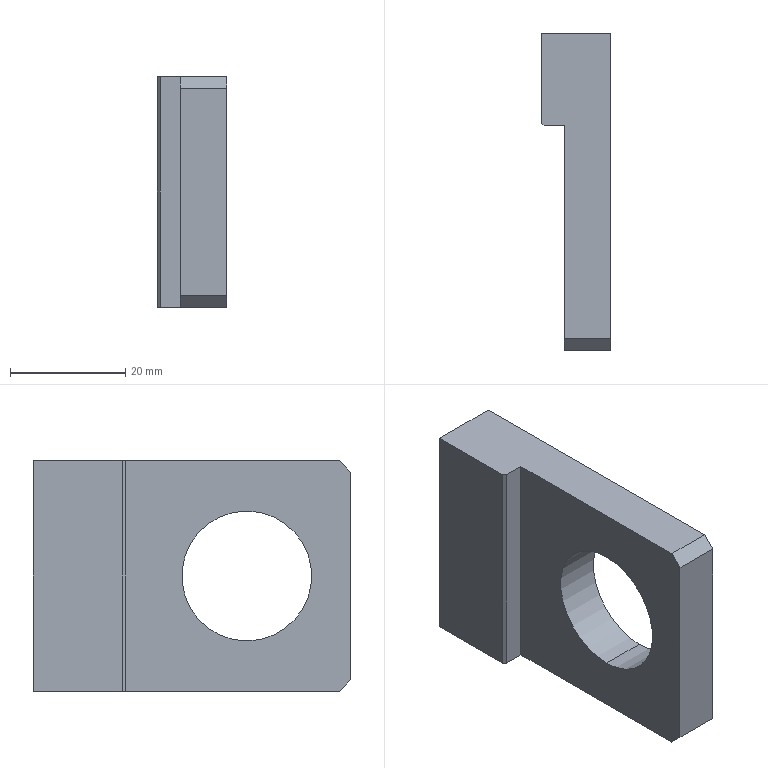Part | STEP file | PN_0027 | 1 solid | 21 faces | box 12 x 55 x 40 mm | volume 16587 mm3 | plane 11 | cylinder 6 | cone 4 | commonest cylinder face diameters 4.2 x4 22.5 x2
STEP:
#1=CARTESIAN_POINT('',(0.,0.,0.));
#2=DIRECTION('',(0.,0.,1.));
#3=DIRECTION('',(1.,0.,0.));
#4=AXIS2_PLACEMENT_3D('',#1,#2,#3);
#5=CARTESIAN_POINT('',(0.,-12.4,16.1));
#6=VERTEX_POINT('',#5);
#7=CARTESIAN_POINT('',(0.,0.,16.1));
#8=VERTEX_POINT('',#7);
#9=CARTESIAN_POINT('',(0.,0.,16.1));
#10=DIRECTION('',(0.,1.,0.));
#11=VECTOR('',#10,1.);
#12=LINE('',#9,#11);
#13=CARTESIAN_POINT('',(0.,0.,14.));
#14=DIRECTION('',(0.,1.,0.));
#15=DIRECTION('',(0.,0.,1.));
#16=AXIS2_PLACEMENT_3D('',#13,#14,#15);
#17=CYLINDRICAL_SURFACE('',#16,2.1);
#18=CARTESIAN_POINT('',(6.283,0.));
#19=DIRECTION('',(0.,1.));
#20=VECTOR('',#19,1.);
#21=LINE('',#18,#20);
#22=(GEOMETRIC_REPRESENTATION_CONTEXT(2)PARAMETRIC_REPRESENTATION_CONTEXT()REPRESENTATION_CONTEXT('',''));
#23=DEFINITIONAL_REPRESENTATION('',(#21),#22);
#24=PCURVE('',#17,#23);
#25=CARTESIAN_POINT('',(0.,0.,14.));
#26=DIRECTION('',(0.,1.,0.));
#27=DIRECTION('',(0.,0.,1.));
#28=AXIS2_PLACEMENT_3D('',#25,#26,#27);
#29=CYLINDRICAL_SURFACE('',#28,2.1);
#30=CARTESIAN_POINT('',(0.,0.));
#31=DIRECTION('',(0.,1.));
#32=VECTOR('',#31,1.);
#33=LINE('',#30,#32);
#34=(GEOMETRIC_REPRESENTATION_CONTEXT(2)PARAMETRIC_REPRESENTATION_CONTEXT()REPRESENTATION_CONTEXT('',''));
#35=DEFINITIONAL_REPRESENTATION('',(#33),#34);
#36=PCURVE('',#29,#35);
#37=SURFACE_CURVE('',#12,(#24,#36),.PCURVE_S1.);
#38=EDGE_CURVE('',#6,#8,#37,.T.);
#39=ORIENTED_EDGE('',*,*,#38,.T.);
#40=CARTESIAN_POINT('',(0.,0.,11.9));
#41=VERTEX_POINT('',#40);
#42=CARTESIAN_POINT('',(0.,0.,14.));
#43=DIRECTION('',(0.,1.,0.));
#44=DIRECTION('',(0.,0.,1.));
#45=AXIS2_PLACEMENT_3D('',#42,#43,#44);
#46=CIRCLE('',#45,2.1);
#47=CARTESIAN_POINT('',(0.,0.));
#48=DIRECTION('',(1.,0.));
#49=VECTOR('',#48,1.);
#50=LINE('',#47,#49);
#51=(GEOMETRIC_REPRESENTATION_CONTEXT(2)PARAMETRIC_REPRESENTATION_CONTEXT()REPRESENTATION_CONTEXT('',''));
#52=DEFINITIONAL_REPRESENTATION('',(#50),#51);
#53=PCURVE('',#17,#52);
#54=CARTESIAN_POINT('',(0.,0.,0.));
#55=DIRECTION('',(0.,1.,0.));
#56=DIRECTION('',(0.,0.,1.));
#57=AXIS2_PLACEMENT_3D('',#54,#55,#56);
#58=PLANE('',#57);
#59=CARTESIAN_POINT('',(14.,0.));
#60=DIRECTION('',(1.,0.));
#61=AXIS2_PLACEMENT_2D('',#59,#60);
#62=CIRCLE('',#61,2.1);
#63=(GEOMETRIC_REPRESENTATION_CONTEXT(2)PARAMETRIC_REPRESENTATION_CONTEXT()REPRESENTATION_CONTEXT('',''));
#64=DEFINITIONAL_REPRESENTATION('',(#62),#63);
#65=PCURVE('',#58,#64);
#66=SURFACE_CURVE('',#46,(#53,#65),.PCURVE_S1.);
#67=EDGE_CURVE('',#41,#8,#66,.T.);
#68=ORIENTED_EDGE('',*,*,#67,.F.);
#69=CARTESIAN_POINT('',(0.,-12.4,11.9));
#70=VERTEX_POINT('',#69);
#71=CARTESIAN_POINT('',(0.,0.,11.9));
#72=DIRECTION('',(0.,1.,0.));
#73=VECTOR('',#72,1.);
#74=LINE('',#71,#73);
#75=CARTESIAN_POINT('',(3.142,0.));
#76=DIRECTION('',(0.,1.));
#77=VECTOR('',#76,1.);
#78=LINE('',#75,#77);
#79=(GEOMETRIC_REPRESENTATION_CONTEXT(2)PARAMETRIC_REPRESENTATION_CONTEXT()REPRESENTATION_CONTEXT('',''));
#80=DEFINITIONAL_REPRESENTATION('',(#78),#79);
#81=PCURVE('',#17,#80);
#82=CARTESIAN_POINT('',(3.142,0.));
#83=DIRECTION('',(0.,1.));
#84=VECTOR('',#83,1.);
#85=LINE('',#82,#84);
#86=(GEOMETRIC_REPRESENTATION_CONTEXT(2)PARAMETRIC_REPRESENTATION_CONTEXT()REPRESENTATION_CONTEXT('',''));
#87=DEFINITIONAL_REPRESENTATION('',(#85),#86);
#88=PCURVE('',#29,#87);
#89=SURFACE_CURVE('',#74,(#81,#88),.PCURVE_S1.);
#90=EDGE_CURVE('',#70,#41,#89,.T.);
#91=ORIENTED_EDGE('',*,*,#90,.F.);
#92=CARTESIAN_POINT('',(0.,-12.4,14.));
#93=DIRECTION('',(0.,1.,0.));
#94=DIRECTION('',(0.,0.,1.));
#95=AXIS2_PLACEMENT_3D('',#92,#93,#94);
#96=CIRCLE('',#95,2.1);
#97=CARTESIAN_POINT('',(0.,-12.4));
#98=DIRECTION('',(1.,0.));
#99=VECTOR('',#98,1.);
#100=LINE('',#97,#99);
#101=(GEOMETRIC_REPRESENTATION_CONTEXT(2)PARAMETRIC_REPRESENTATION_CONTEXT()REPRESENTATION_CONTEXT('',''));
#102=DEFINITIONAL_REPRESENTATION('',(#100),#101);
#103=PCURVE('',#17,#102);
#104=CARTESIAN_POINT('',(0.,-12.4,14.));
#105=DIRECTION('',(0.,1.,0.));
#106=DIRECTION('',(0.,0.,1.));
#107=AXIS2_PLACEMENT_3D('',#104,#105,#106);
#108=CONICAL_SURFACE('',#107,2.1,1.03);
#109=CARTESIAN_POINT('',(0.,0.));
#110=DIRECTION('',(1.,0.));
#111=VECTOR('',#110,1.);
#112=LINE('',#109,#111);
#113=(GEOMETRIC_REPRESENTATION_CONTEXT(2)PARAMETRIC_REPRESENTATION_CONTEXT()REPRESENTATION_CONTEXT('',''));
#114=DEFINITIONAL_REPRESENTATION('',(#112),#113);
#115=PCURVE('',#108,#114);
#116=SURFACE_CURVE('',#96,(#103,#115),.PCURVE_S1.);
#117=EDGE_CURVE('',#70,#6,#116,.T.);
#118=ORIENTED_EDGE('',*,*,#117,.T.);
#119=EDGE_LOOP('',(#39,#68,#91,#118));
#120=FACE_BOUND('',#119,.F.);
#121=ADVANCED_FACE('',(#120),#17,.F.);
#122=ORIENTED_EDGE('',*,*,#117,.F.);
#123=CARTESIAN_POINT('',(0.,-13.662,14.));
#124=VERTEX_POINT('',#123);
#125=CARTESIAN_POINT('',(0.,-12.4,11.9));
#126=DIRECTION('',(0.,0.515,-0.8572));
#127=VECTOR('',#126,1.);
#128=LINE('',#125,#127);
#129=CARTESIAN_POINT('',(3.142,0.));
#130=DIRECTION('',(0.,1.));
#131=VECTOR('',#130,1.);
#132=LINE('',#129,#131);
#133=(GEOMETRIC_REPRESENTATION_CONTEXT(2)PARAMETRIC_REPRESENTATION_CONTEXT()REPRESENTATION_CONTEXT('',''));
#134=DEFINITIONAL_REPRESENTATION('',(#132),#133);
#135=PCURVE('',#108,#134);
#136=CARTESIAN_POINT('',(0.,-12.4,14.));
#137=DIRECTION('',(0.,1.,0.));
#138=DIRECTION('',(0.,0.,1.));
#139=AXIS2_PLACEMENT_3D('',#136,#137,#138);
#140=CONICAL_SURFACE('',#139,2.1,1.03);
#141=CARTESIAN_POINT('',(3.142,0.));
#142=DIRECTION('',(0.,1.));
#143=VECTOR('',#142,1.);
#144=LINE('',#141,#143);
#145=(GEOMETRIC_REPRESENTATION_CONTEXT(2)PARAMETRIC_REPRESENTATION_CONTEXT()REPRESENTATION_CONTEXT('',''));
#146=DEFINITIONAL_REPRESENTATION('',(#144),#145);
#147=PCURVE('',#140,#146);
#148=SURFACE_CURVE('',#128,(#135,#147),.PCURVE_S1.);
#149=EDGE_CURVE('',#124,#70,#148,.T.);
#150=ORIENTED_EDGE('',*,*,#149,.F.);
#151=CARTESIAN_POINT('',(0.,-12.4,16.1));
#152=DIRECTION('',(0.,0.515,0.8572));
#153=VECTOR('',#152,1.);
#154=LINE('',#151,#153);
#155=CARTESIAN_POINT('',(6.283,0.));
#156=DIRECTION('',(0.,1.));
#157=VECTOR('',#156,1.);
#158=LINE('',#155,#157);
#159=(GEOMETRIC_REPRESENTATION_CONTEXT(2)PARAMETRIC_REPRESENTATION_CONTEXT()REPRESENTATION_CONTEXT('',''));
#160=DEFINITIONAL_REPRESENTATION('',(#158),#159);
#161=PCURVE('',#108,#160);
#162=CARTESIAN_POINT('',(0.,0.));
#163=DIRECTION('',(0.,1.));
#164=VECTOR('',#163,1.);
#165=LINE('',#162,#164);
#166=(GEOMETRIC_REPRESENTATION_CONTEXT(2)PARAMETRIC_REPRESENTATION_CONTEXT()REPRESENTATION_CONTEXT('',''));
#167=DEFINITIONAL_REPRESENTATION('',(#165),#166);
#168=PCURVE('',#140,#167);
#169=SURFACE_CURVE('',#154,(#161,#168),.PCURVE_S1.);
#170=EDGE_CURVE('',#124,#6,#169,.T.);
#171=ORIENTED_EDGE('',*,*,#170,.T.);
#172=EDGE_LOOP('',(#122,#150,#171));
#173=FACE_BOUND('',#172,.F.);
#174=ADVANCED_FACE('',(#173),#108,.F.);
#175=CARTESIAN_POINT('',(0.,-12.4,-11.9));
#176=VERTEX_POINT('',#175);
#177=CARTESIAN_POINT('',(0.,0.,-11.9));
#178=VERTEX_POINT('',#177);
#179=CARTESIAN_POINT('',(0.,0.,-11.9));
#180=DIRECTION('',(0.,1.,0.));
#181=VECTOR('',#180,1.);
#182=LINE('',#179,#181);
#183=CARTESIAN_POINT('',(0.,0.,-14.));
#184=DIRECTION('',(0.,1.,0.));
#185=DIRECTION('',(0.,0.,1.));
#186=AXIS2_PLACEMENT_3D('',#183,#184,#185);
#187=CYLINDRICAL_SURFACE('',#186,2.1);
#188=CARTESIAN_POINT('',(6.283,0.));
#189=DIRECTION('',(0.,1.));
#190=VECTOR('',#189,1.);
#191=LINE('',#188,#190);
#192=(GEOMETRIC_REPRESENTATION_CONTEXT(2)PARAMETRIC_REPRESENTATION_CONTEXT()REPRESENTATION_CONTEXT('',''));
#193=DEFINITIONAL_REPRESENTATION('',(#191),#192);
#194=PCURVE('',#187,#193);
#195=CARTESIAN_POINT('',(0.,0.,-14.));
#196=DIRECTION('',(0.,1.,0.));
#197=DIRECTION('',(0.,0.,1.));
#198=AXIS2_PLACEMENT_3D('',#195,#196,#197);
#199=CYLINDRICAL_SURFACE('',#198,2.1);
#200=CARTESIAN_POINT('',(0.,0.));
#201=DIRECTION('',(0.,1.));
#202=VECTOR('',#201,1.);
#203=LINE('',#200,#202);
#204=(GEOMETRIC_REPRESENTATION_CONTEXT(2)PARAMETRIC_REPRESENTATION_CONTEXT()REPRESENTATION_CONTEXT('',''));
#205=DEFINITIONAL_REPRESENTATION('',(#203),#204);
#206=PCURVE('',#199,#205);
#207=SURFACE_CURVE('',#182,(#194,#206),.PCURVE_S1.);
#208=EDGE_CURVE('',#176,#178,#207,.T.);
#209=ORIENTED_EDGE('',*,*,#208,.T.);
#210=CARTESIAN_POINT('',(0.,0.,-16.1));
#211=VERTEX_POINT('',#210);
#212=CARTESIAN_POINT('',(0.,0.,-14.));
#213=DIRECTION('',(0.,1.,0.));
#214=DIRECTION('',(0.,0.,1.));
#215=AXIS2_PLACEMENT_3D('',#212,#213,#214);
#216=CIRCLE('',#215,2.1);
#217=CARTESIAN_POINT('',(0.,0.));
#218=DIRECTION('',(1.,0.));
#219=VECTOR('',#218,1.);
#220=LINE('',#217,#219);
#221=(GEOMETRIC_REPRESENTATION_CONTEXT(2)PARAMETRIC_REPRESENTATION_CONTEXT()REPRESENTATION_CONTEXT('',''));
#222=DEFINITIONAL_REPRESENTATION('',(#220),#221);
#223=PCURVE('',#187,#222);
#224=CARTESIAN_POINT('',(-14.,0.));
#225=DIRECTION('',(1.,0.));
#226=AXIS2_PLACEMENT_2D('',#224,#225);
#227=CIRCLE('',#226,2.1);
#228=(GEOMETRIC_REPRESENTATION_CONTEXT(2)PARAMETRIC_REPRESENTATION_CONTEXT()REPRESENTATION_CONTEXT('',''));
#229=DEFINITIONAL_REPRESENTATION('',(#227),#228);
#230=PCURVE('',#58,#229);
#231=SURFACE_CURVE('',#216,(#223,#230),.PCURVE_S1.);
#232=EDGE_CURVE('',#211,#178,#231,.T.);
#233=ORIENTED_EDGE('',*,*,#232,.F.);
#234=CARTESIAN_POINT('',(0.,-12.4,-16.1));
#235=VERTEX_POINT('',#234);
#236=CARTESIAN_POINT('',(0.,0.,-16.1));
#237=DIRECTION('',(0.,1.,0.));
#238=VECTOR('',#237,1.);
#239=LINE('',#236,#238);
#240=CARTESIAN_POINT('',(3.142,0.));
#241=DIRECTION('',(0.,1.));
#242=VECTOR('',#241,1.);
#243=LINE('',#240,#242);
#244=(GEOMETRIC_REPRESENTATION_CONTEXT(2)PARAMETRIC_REPRESENTATION_CONTEXT()REPRESENTATION_CONTEXT('',''));
#245=DEFINITIONAL_REPRESENTATION('',(#243),#244);
#246=PCURVE('',#187,#245);
#247=CARTESIAN_POINT('',(3.142,0.));
#248=DIRECTION('',(0.,1.));
#249=VECTOR('',#248,1.);
#250=LINE('',#247,#249);
#251=(GEOMETRIC_REPRESENTATION_CONTEXT(2)PARAMETRIC_REPRESENTATION_CONTEXT()REPRESENTATION_CONTEXT('',''));
#252=DEFINITIONAL_REPRESENTATION('',(#250),#251);
#253=PCURVE('',#199,#252);
#254=SURFACE_CURVE('',#239,(#246,#253),.PCURVE_S1.);
#255=EDGE_CURVE('',#235,#211,#254,.T.);
#256=ORIENTED_EDGE('',*,*,#255,.F.);
#257=CARTESIAN_POINT('',(0.,-12.4,-14.));
#258=DIRECTION('',(0.,1.,0.));
#259=DIRECTION('',(0.,0.,1.));
#260=AXIS2_PLACEMENT_3D('',#257,#258,#259);
#261=CIRCLE('',#260,2.1);
#262=CARTESIAN_POINT('',(0.,-12.4));
#263=DIRECTION('',(1.,0.));
#264=VECTOR('',#263,1.);
#265=LINE('',#262,#264);
#266=(GEOMETRIC_REPRESENTATION_CONTEXT(2)PARAMETRIC_REPRESENTATION_CONTEXT()REPRESENTATION_CONTEXT('',''));
#267=DEFINITIONAL_REPRESENTATION('',(#265),#266);
#268=PCURVE('',#187,#267);
#269=CARTESIAN_POINT('',(0.,-12.4,-14.));
#270=DIRECTION('',(0.,1.,0.));
#271=DIRECTION('',(0.,0.,1.));
#272=AXIS2_PLACEMENT_3D('',#269,#270,#271);
#273=CONICAL_SURFACE('',#272,2.1,1.03);
#274=CARTESIAN_POINT('',(0.,0.));
#275=DIRECTION('',(1.,0.));
#276=VECTOR('',#275,1.);
#277=LINE('',#274,#276);
#278=(GEOMETRIC_REPRESENTATION_CONTEXT(2)PARAMETRIC_REPRESENTATION_CONTEXT()REPRESENTATION_CONTEXT('',''));
#279=DEFINITIONAL_REPRESENTATION('',(#277),#278);
#280=PCURVE('',#273,#279);
#281=SURFACE_CURVE('',#261,(#268,#280),.PCURVE_S1.);
#282=EDGE_CURVE('',#235,#176,#281,.T.);
#283=ORIENTED_EDGE('',*,*,#282,.T.);
#284=EDGE_LOOP('',(#209,#233,#256,#283));
#285=FACE_BOUND('',#284,.F.);
#286=ADVANCED_FACE('',(#285),#187,.F.);
#287=ORIENTED_EDGE('',*,*,#282,.F.);
#288=CARTESIAN_POINT('',(0.,-13.662,-14.));
#289=VERTEX_POINT('',#288);
#290=CARTESIAN_POINT('',(0.,-12.4,-16.1));
#291=DIRECTION('',(0.,0.515,-0.8572));
#292=VECTOR('',#291,1.);
#293=LINE('',#290,#292);
#294=CARTESIAN_POINT('',(3.142,0.));
#295=DIRECTION('',(0.,1.));
#296=VECTOR('',#295,1.);
#297=LINE('',#294,#296);
#298=(GEOMETRIC_REPRESENTATION_CONTEXT(2)PARAMETRIC_REPRESENTATION_CONTEXT()REPRESENTATION_CONTEXT('',''));
#299=DEFINITIONAL_REPRESENTATION('',(#297),#298);
#300=PCURVE('',#273,#299);
#301=CARTESIAN_POINT('',(0.,-12.4,-14.));
#302=DIRECTION('',(0.,1.,0.));
#303=DIRECTION('',(0.,0.,1.));
#304=AXIS2_PLACEMENT_3D('',#301,#302,#303);
#305=CONICAL_SURFACE('',#304,2.1,1.03);
#306=CARTESIAN_POINT('',(3.142,0.));
#307=DIRECTION('',(0.,1.));
#308=VECTOR('',#307,1.);
#309=LINE('',#306,#308);
#310=(GEOMETRIC_REPRESENTATION_CONTEXT(2)PARAMETRIC_REPRESENTATION_CONTEXT()REPRESENTATION_CONTEXT('',''));
#311=DEFINITIONAL_REPRESENTATION('',(#309),#310);
#312=PCURVE('',#305,#311);
#313=SURFACE_CURVE('',#293,(#300,#312),.PCURVE_S1.);
#314=EDGE_CURVE('',#289,#235,#313,.T.);
#315=ORIENTED_EDGE('',*,*,#314,.F.);
#316=CARTESIAN_POINT('',(0.,-12.4,-11.9));
#317=DIRECTION('',(0.,0.515,0.8572));
#318=VECTOR('',#317,1.);
#319=LINE('',#316,#318);
#320=CARTESIAN_POINT('',(6.283,0.));
#321=DIRECTION('',(0.,1.));
#322=VECTOR('',#321,1.);
#323=LINE('',#320,#322);
#324=(GEOMETRIC_REPRESENTATION_CONTEXT(2)PARAMETRIC_REPRESENTATION_CONTEXT()REPRESENTATION_CONTEXT('',''));
#325=DEFINITIONAL_REPRESENTATION('',(#323),#324);
#326=PCURVE('',#273,#325);
#327=CARTESIAN_POINT('',(0.,0.));
#328=DIRECTION('',(0.,1.));
#329=VECTOR('',#328,1.);
#330=LINE('',#327,#329);
#331=(GEOMETRIC_REPRESENTATION_CONTEXT(2)PARAMETRIC_REPRESENTATION_CONTEXT()REPRESENTATION_CONTEXT('',''));
#332=DEFINITIONAL_REPRESENTATION('',(#330),#331);
#333=PCURVE('',#305,#332);
#334=SURFACE_CURVE('',#319,(#326,#333),.PCURVE_S1.);
#335=EDGE_CURVE('',#289,#176,#334,.T.);
#336=ORIENTED_EDGE('',*,*,#335,.T.);
#337=EDGE_LOOP('',(#287,#315,#336));
#338=FACE_BOUND('',#337,.F.);
#339=ADVANCED_FACE('',(#338),#273,.F.);
#340=CARTESIAN_POINT('',(-2.,-37.,-11.25));
#341=VERTEX_POINT('',#340);
#342=CARTESIAN_POINT('',(6.,-37.,-11.25));
#343=VERTEX_POINT('',#342);
#344=CARTESIAN_POINT('',(-6.,-37.,-11.25));
#345=DIRECTION('',(1.,0.,0.));
#346=VECTOR('',#345,1.);
#347=LINE('',#344,#346);
#348=CARTESIAN_POINT('',(-6.,-37.,0.));
#349=DIRECTION('',(1.,0.,0.));
#350=DIRECTION('',(0.,0.,-1.));
#351=AXIS2_PLACEMENT_3D('',#348,#349,#350);
#352=CYLINDRICAL_SURFACE('',#351,11.25);
#353=CARTESIAN_POINT('',(6.283,0.));
#354=DIRECTION('',(0.,1.));
#355=VECTOR('',#354,1.);
#356=LINE('',#353,#355);
#357=(GEOMETRIC_REPRESENTATION_CONTEXT(2)PARAMETRIC_REPRESENTATION_CONTEXT()REPRESENTATION_CONTEXT('',''));
#358=DEFINITIONAL_REPRESENTATION('',(#356),#357);
#359=PCURVE('',#352,#358);
#360=CARTESIAN_POINT('',(-6.,-37.,0.));
#361=DIRECTION('',(1.,0.,0.));
#362=DIRECTION('',(0.,0.,-1.));
#363=AXIS2_PLACEMENT_3D('',#360,#361,#362);
#364=CYLINDRICAL_SURFACE('',#363,11.25);
#365=CARTESIAN_POINT('',(0.,0.));
#366=DIRECTION('',(0.,1.));
#367=VECTOR('',#366,1.);
#368=LINE('',#365,#367);
#369=(GEOMETRIC_REPRESENTATION_CONTEXT(2)PARAMETRIC_REPRESENTATION_CONTEXT()REPRESENTATION_CONTEXT('',''));
#370=DEFINITIONAL_REPRESENTATION('',(#368),#369);
#371=PCURVE('',#364,#370);
#372=SURFACE_CURVE('',#347,(#359,#371),.PCURVE_S1.);
#373=EDGE_CURVE('',#341,#343,#372,.T.);
#374=ORIENTED_EDGE('',*,*,#373,.T.);
#375=CARTESIAN_POINT('',(6.,-37.,11.25));
#376=VERTEX_POINT('',#375);
#377=CARTESIAN_POINT('',(6.,-37.,0.));
#378=DIRECTION('',(1.,0.,0.));
#379=DIRECTION('',(0.,0.,-1.));
#380=AXIS2_PLACEMENT_3D('',#377,#378,#379);
#381=CIRCLE('',#380,11.25);
#382=CARTESIAN_POINT('',(0.,12.));
#383=DIRECTION('',(1.,0.));
#384=VECTOR('',#383,1.);
#385=LINE('',#382,#384);
#386=(GEOMETRIC_REPRESENTATION_CONTEXT(2)PARAMETRIC_REPRESENTATION_CONTEXT()REPRESENTATION_CONTEXT('',''));
#387=DEFINITIONAL_REPRESENTATION('',(#385),#386);
#388=PCURVE('',#352,#387);
#389=CARTESIAN_POINT('',(6.,-55.,-20.));
#390=DIRECTION('',(1.,0.,0.));
#391=DIRECTION('',(0.,0.,-1.));
#392=AXIS2_PLACEMENT_3D('',#389,#390,#391);
#393=PLANE('',#392);
#394=CARTESIAN_POINT('',(-20.,18.));
#395=DIRECTION('',(1.,0.));
#396=AXIS2_PLACEMENT_2D('',#394,#395);
#397=CIRCLE('',#396,11.25);
#398=(GEOMETRIC_REPRESENTATION_CONTEXT(2)PARAMETRIC_REPRESENTATION_CONTEXT()REPRESENTATION_CONTEXT('',''));
#399=DEFINITIONAL_REPRESENTATION('',(#397),#398);
#400=PCURVE('',#393,#399);
#401=SURFACE_CURVE('',#381,(#388,#400),.PCURVE_S1.);
#402=EDGE_CURVE('',#376,#343,#401,.T.);
#403=ORIENTED_EDGE('',*,*,#402,.F.);
#404=CARTESIAN_POINT('',(-2.,-37.,11.25));
#405=VERTEX_POINT('',#404);
#406=CARTESIAN_POINT('',(-6.,-37.,11.25));
#407=DIRECTION('',(1.,0.,0.));
#408=VECTOR('',#407,1.);
#409=LINE('',#406,#408);
#410=CARTESIAN_POINT('',(3.142,0.));
#411=DIRECTION('',(0.,1.));
#412=VECTOR('',#411,1.);
#413=LINE('',#410,#412);
#414=(GEOMETRIC_REPRESENTATION_CONTEXT(2)PARAMETRIC_REPRESENTATION_CONTEXT()REPRESENTATION_CONTEXT('',''));
#415=DEFINITIONAL_REPRESENTATION('',(#413),#414);
#416=PCURVE('',#352,#415);
#417=CARTESIAN_POINT('',(3.142,0.));
#418=DIRECTION('',(0.,1.));
#419=VECTOR('',#418,1.);
#420=LINE('',#417,#419);
#421=(GEOMETRIC_REPRESENTATION_CONTEXT(2)PARAMETRIC_REPRESENTATION_CONTEXT()REPRESENTATION_CONTEXT('',''));
#422=DEFINITIONAL_REPRESENTATION('',(#420),#421);
#423=PCURVE('',#364,#422);
#424=SURFACE_CURVE('',#409,(#416,#423),.PCURVE_S1.);
#425=EDGE_CURVE('',#405,#376,#424,.T.);
#426=ORIENTED_EDGE('',*,*,#425,.F.);
#427=CARTESIAN_POINT('',(-2.,-37.,0.));
#428=DIRECTION('',(-1.,0.,0.));
#429=DIRECTION('',(0.,0.,-1.));
#430=AXIS2_PLACEMENT_3D('',#427,#428,#429);
#431=CIRCLE('',#430,11.25);
#432=CARTESIAN_POINT('',(6.283,4.));
#433=DIRECTION('',(-1.,0.));
#434=VECTOR('',#433,1.);
#435=LINE('',#432,#434);
#436=(GEOMETRIC_REPRESENTATION_CONTEXT(2)PARAMETRIC_REPRESENTATION_CONTEXT()REPRESENTATION_CONTEXT('',''));
#437=DEFINITIONAL_REPRESENTATION('',(#435),#436);
#438=PCURVE('',#352,#437);
#439=CARTESIAN_POINT('',(-2.,-55.,-20.));
#440=DIRECTION('',(1.,0.,0.));
#441=DIRECTION('',(0.,0.,-1.));
#442=AXIS2_PLACEMENT_3D('',#439,#440,#441);
#443=PLANE('',#442);
#444=CARTESIAN_POINT('',(-8.75,18.));
#445=CARTESIAN_POINT('',(-8.75,-1.486));
#446=CARTESIAN_POINT('',(-25.625,8.257));
#447=CARTESIAN_POINT('',(-42.5,18.));
#448=CARTESIAN_POINT('',(-25.625,27.743));
#449=CARTESIAN_POINT('',(-8.75,37.486));
#450=CARTESIAN_POINT('',(-8.75,18.));
#451=(BOUNDED_CURVE()B_SPLINE_CURVE(2,(#444,#445,#446,#447,#448,#449,#450),.UNSPECIFIED.,.T.,.F.)B_SPLINE_CURVE_WITH_KNOTS((1,2,2,2,2,1),(-2.094,0.,2.094,4.189,6.283,8.378),.UNSPECIFIED.)CURVE()GEOMETRIC_REPRESENTATION_ITEM()RATIONAL_B_SPLINE_CURVE((1.,0.5,1.,0.5,1.,0.5,1.))REPRESENTATION_ITEM(''));
#452=(GEOMETRIC_REPRESENTATION_CONTEXT(2)PARAMETRIC_REPRESENTATION_CONTEXT()REPRESENTATION_CONTEXT('',''));
#453=DEFINITIONAL_REPRESENTATION('',(#451),#452);
#454=PCURVE('',#443,#453);
#455=SURFACE_CURVE('',#431,(#438,#454),.PCURVE_S1.);
#456=EDGE_CURVE('',#341,#405,#455,.T.);
#457=ORIENTED_EDGE('',*,*,#456,.F.);
#458=EDGE_LOOP('',(#374,#403,#426,#457));
#459=FACE_BOUND('',#458,.F.);
#460=ADVANCED_FACE('',(#459),#352,.F.);
#461=CARTESIAN_POINT('',(6.,-37.,0.));
#462=DIRECTION('',(1.,0.,0.));
#463=DIRECTION('',(0.,0.,-1.));
#464=AXIS2_PLACEMENT_3D('',#461,#462,#463);
#465=CIRCLE('',#464,11.25);
#466=CARTESIAN_POINT('',(-20.,18.));
#467=DIRECTION('',(1.,0.));
#468=AXIS2_PLACEMENT_2D('',#466,#467);
#469=CIRCLE('',#468,11.25);
#470=(GEOMETRIC_REPRESENTATION_CONTEXT(2)PARAMETRIC_REPRESENTATION_CONTEXT()REPRESENTATION_CONTEXT('',''));
#471=DEFINITIONAL_REPRESENTATION('',(#469),#470);
#472=PCURVE('',#393,#471);
#473=CARTESIAN_POINT('',(0.,12.));
#474=DIRECTION('',(1.,0.));
#475=VECTOR('',#474,1.);
#476=LINE('',#473,#475);
#477=(GEOMETRIC_REPRESENTATION_CONTEXT(2)PARAMETRIC_REPRESENTATION_CONTEXT()REPRESENTATION_CONTEXT('',''));
#478=DEFINITIONAL_REPRESENTATION('',(#476),#477);
#479=PCURVE('',#364,#478);
#480=SURFACE_CURVE('',#465,(#472,#479),.PCURVE_S1.);
#481=EDGE_CURVE('',#343,#376,#480,.T.);
#482=ORIENTED_EDGE('',*,*,#481,.F.);
#483=ORIENTED_EDGE('',*,*,#402,.F.);
#484=EDGE_LOOP('',(#482,#483));
#485=FACE_BOUND('',#484,.T.);
#486=CARTESIAN_POINT('',(6.,-55.,18.));
#487=VERTEX_POINT('',#486);
#488=CARTESIAN_POINT('',(6.,-55.,-18.));
#489=VERTEX_POINT('',#488);
#490=CARTESIAN_POINT('',(6.,-55.,-20.));
#491=DIRECTION('',(0.,0.,-1.));
#492=VECTOR('',#491,1.);
#493=LINE('',#490,#492);
#494=CARTESIAN_POINT('',(0.,0.));
#495=DIRECTION('',(1.,0.));
#496=VECTOR('',#495,1.);
#497=LINE('',#494,#496);
#498=(GEOMETRIC_REPRESENTATION_CONTEXT(2)PARAMETRIC_REPRESENTATION_CONTEXT()REPRESENTATION_CONTEXT('',''));
#499=DEFINITIONAL_REPRESENTATION('',(#497),#498);
#500=PCURVE('',#393,#499);
#501=CARTESIAN_POINT('',(0.,-55.,0.));
#502=DIRECTION('',(0.,1.,0.));
#503=DIRECTION('',(0.,0.,1.));
#504=AXIS2_PLACEMENT_3D('',#501,#502,#503);
#505=PLANE('',#504);
#506=CARTESIAN_POINT('',(-20.,6.));
#507=DIRECTION('',(-1.,0.));
#508=VECTOR('',#507,1.);
#509=LINE('',#506,#508);
#510=(GEOMETRIC_REPRESENTATION_CONTEXT(2)PARAMETRIC_REPRESENTATION_CONTEXT()REPRESENTATION_CONTEXT('',''));
#511=DEFINITIONAL_REPRESENTATION('',(#509),#510);
#512=PCURVE('',#505,#511);
#513=SURFACE_CURVE('',#493,(#500,#512),.PCURVE_S1.);
#514=EDGE_CURVE('',#487,#489,#513,.T.);
#515=ORIENTED_EDGE('',*,*,#514,.T.);
#516=CARTESIAN_POINT('',(6.,-53.,-20.));
#517=VERTEX_POINT('',#516);
#518=CARTESIAN_POINT('',(6.,-54.,-19.));
#519=DIRECTION('',(0.,0.7071,-0.7071));
#520=VECTOR('',#519,1.);
#521=LINE('',#518,#520);
#522=CARTESIAN_POINT('',(-1.,1.));
#523=DIRECTION('',(0.7071,0.7071));
#524=VECTOR('',#523,1.);
#525=LINE('',#522,#524);
#526=(GEOMETRIC_REPRESENTATION_CONTEXT(2)PARAMETRIC_REPRESENTATION_CONTEXT()REPRESENTATION_CONTEXT('',''));
#527=DEFINITIONAL_REPRESENTATION('',(#525),#526);
#528=PCURVE('',#393,#527);
#529=CARTESIAN_POINT('',(-6.,-53.,-20.));
#530=DIRECTION('',(0.,-0.7071,-0.7071));
#531=DIRECTION('',(1.,0.,0.));
#532=AXIS2_PLACEMENT_3D('',#529,#530,#531);
#533=PLANE('',#532);
#534=CARTESIAN_POINT('',(12.,1.414));
#535=DIRECTION('',(0.,-1.));
#536=VECTOR('',#535,1.);
#537=LINE('',#534,#536);
#538=(GEOMETRIC_REPRESENTATION_CONTEXT(2)PARAMETRIC_REPRESENTATION_CONTEXT()REPRESENTATION_CONTEXT('',''));
#539=DEFINITIONAL_REPRESENTATION('',(#537),#538);
#540=PCURVE('',#533,#539);
#541=SURFACE_CURVE('',#521,(#528,#540),.PCURVE_S1.);
#542=EDGE_CURVE('',#489,#517,#541,.T.);
#543=ORIENTED_EDGE('',*,*,#542,.T.);
#544=CARTESIAN_POINT('',(6.,0.,-20.));
#545=VERTEX_POINT('',#544);
#546=CARTESIAN_POINT('',(6.,-55.,-20.));
#547=DIRECTION('',(0.,1.,0.));
#548=VECTOR('',#547,1.);
#549=LINE('',#546,#548);
#550=CARTESIAN_POINT('',(0.,0.));
#551=DIRECTION('',(0.,1.));
#552=VECTOR('',#551,1.);
#553=LINE('',#550,#552);
#554=(GEOMETRIC_REPRESENTATION_CONTEXT(2)PARAMETRIC_REPRESENTATION_CONTEXT()REPRESENTATION_CONTEXT('',''));
#555=DEFINITIONAL_REPRESENTATION('',(#553),#554);
#556=PCURVE('',#393,#555);
#557=CARTESIAN_POINT('',(-6.,-55.,-20.));
#558=DIRECTION('',(0.,0.,-1.));
#559=DIRECTION('',(-1.,0.,0.));
#560=AXIS2_PLACEMENT_3D('',#557,#558,#559);
#561=PLANE('',#560);
#562=CARTESIAN_POINT('',(-12.,0.));
#563=DIRECTION('',(0.,1.));
#564=VECTOR('',#563,1.);
#565=LINE('',#562,#564);
#566=(GEOMETRIC_REPRESENTATION_CONTEXT(2)PARAMETRIC_REPRESENTATION_CONTEXT()REPRESENTATION_CONTEXT('',''));
#567=DEFINITIONAL_REPRESENTATION('',(#565),#566);
#568=PCURVE('',#561,#567);
#569=SURFACE_CURVE('',#549,(#556,#568),.PCURVE_S1.);
#570=EDGE_CURVE('',#517,#545,#569,.T.);
#571=ORIENTED_EDGE('',*,*,#570,.T.);
#572=CARTESIAN_POINT('',(6.,0.,20.));
#573=VERTEX_POINT('',#572);
#574=CARTESIAN_POINT('',(6.,0.,-20.));
#575=DIRECTION('',(0.,0.,-1.));
#576=VECTOR('',#575,1.);
#577=LINE('',#574,#576);
#578=CARTESIAN_POINT('',(0.,55.));
#579=DIRECTION('',(1.,0.));
#580=VECTOR('',#579,1.);
#581=LINE('',#578,#580);
#582=(GEOMETRIC_REPRESENTATION_CONTEXT(2)PARAMETRIC_REPRESENTATION_CONTEXT()REPRESENTATION_CONTEXT('',''));
#583=DEFINITIONAL_REPRESENTATION('',(#581),#582);
#584=PCURVE('',#393,#583);
#585=CARTESIAN_POINT('',(-20.,6.));
#586=DIRECTION('',(-1.,0.));
#587=VECTOR('',#586,1.);
#588=LINE('',#585,#587);
#589=(GEOMETRIC_REPRESENTATION_CONTEXT(2)PARAMETRIC_REPRESENTATION_CONTEXT()REPRESENTATION_CONTEXT('',''));
#590=DEFINITIONAL_REPRESENTATION('',(#588),#589);
#591=PCURVE('',#58,#590);
#592=SURFACE_CURVE('',#577,(#584,#591),.PCURVE_S1.);
#593=EDGE_CURVE('',#573,#545,#592,.T.);
#594=ORIENTED_EDGE('',*,*,#593,.F.);
#595=CARTESIAN_POINT('',(6.,-53.,20.));
#596=VERTEX_POINT('',#595);
#597=CARTESIAN_POINT('',(6.,-55.,20.));
#598=DIRECTION('',(0.,1.,0.));
#599=VECTOR('',#598,1.);
#600=LINE('',#597,#599);
#601=CARTESIAN_POINT('',(-40.,0.));
#602=DIRECTION('',(0.,1.));
#603=VECTOR('',#602,1.);
#604=LINE('',#601,#603);
#605=(GEOMETRIC_REPRESENTATION_CONTEXT(2)PARAMETRIC_REPRESENTATION_CONTEXT()REPRESENTATION_CONTEXT('',''));
#606=DEFINITIONAL_REPRESENTATION('',(#604),#605);
#607=PCURVE('',#393,#606);
#608=CARTESIAN_POINT('',(-6.,-55.,20.));
#609=DIRECTION('',(0.,0.,1.));
#610=DIRECTION('',(1.,0.,0.));
#611=AXIS2_PLACEMENT_3D('',#608,#609,#610);
#612=PLANE('',#611);
#613=CARTESIAN_POINT('',(12.,0.));
#614=DIRECTION('',(0.,1.));
#615=VECTOR('',#614,1.);
#616=LINE('',#613,#615);
#617=(GEOMETRIC_REPRESENTATION_CONTEXT(2)PARAMETRIC_REPRESENTATION_CONTEXT()REPRESENTATION_CONTEXT('',''));
#618=DEFINITIONAL_REPRESENTATION('',(#616),#617);
#619=PCURVE('',#612,#618);
#620=SURFACE_CURVE('',#600,(#607,#619),.PCURVE_S1.);
#621=EDGE_CURVE('',#596,#573,#620,.T.);
#622=ORIENTED_EDGE('',*,*,#621,.F.);
#623=CARTESIAN_POINT('',(6.,-74.,-1.));
#624=DIRECTION('',(0.,-0.7071,-0.7071));
#625=VECTOR('',#624,1.);
#626=LINE('',#623,#625);
#627=CARTESIAN_POINT('',(-19.,-19.));
#628=DIRECTION('',(0.7071,-0.7071));
#629=VECTOR('',#628,1.);
#630=LINE('',#627,#629);
#631=(GEOMETRIC_REPRESENTATION_CONTEXT(2)PARAMETRIC_REPRESENTATION_CONTEXT()REPRESENTATION_CONTEXT('',''));
#632=DEFINITIONAL_REPRESENTATION('',(#630),#631);
#633=PCURVE('',#393,#632);
#634=CARTESIAN_POINT('',(-6.,-53.,20.));
#635=DIRECTION('',(0.,-0.7071,0.7071));
#636=DIRECTION('',(-1.,0.,0.));
#637=AXIS2_PLACEMENT_3D('',#634,#635,#636);
#638=PLANE('',#637);
#639=CARTESIAN_POINT('',(-12.,29.698));
#640=DIRECTION('',(0.,1.));
#641=VECTOR('',#640,1.);
#642=LINE('',#639,#641);
#643=(GEOMETRIC_REPRESENTATION_CONTEXT(2)PARAMETRIC_REPRESENTATION_CONTEXT()REPRESENTATION_CONTEXT('',''));
#644=DEFINITIONAL_REPRESENTATION('',(#642),#643);
#645=PCURVE('',#638,#644);
#646=SURFACE_CURVE('',#626,(#633,#645),.PCURVE_S1.);
#647=EDGE_CURVE('',#596,#487,#646,.T.);
#648=ORIENTED_EDGE('',*,*,#647,.T.);
#649=EDGE_LOOP('',(#515,#543,#571,#594,#622,#648));
#650=FACE_BOUND('',#649,.T.);
#651=ADVANCED_FACE('',(#485,#650),#393,.T.);
#652=CARTESIAN_POINT('',(-6.,-15.5,20.));
#653=VERTEX_POINT('',#652);
#654=CARTESIAN_POINT('',(-6.,0.,20.));
#655=VERTEX_POINT('',#654);
#656=CARTESIAN_POINT('',(-6.,-55.,20.));
#657=DIRECTION('',(0.,1.,0.));
#658=VECTOR('',#657,1.);
#659=LINE('',#656,#658);
#660=CARTESIAN_POINT('',(0.,0.));
#661=DIRECTION('',(0.,1.));
#662=VECTOR('',#661,1.);
#663=LINE('',#660,#662);
#664=(GEOMETRIC_REPRESENTATION_CONTEXT(2)PARAMETRIC_REPRESENTATION_CONTEXT()REPRESENTATION_CONTEXT('',''));
#665=DEFINITIONAL_REPRESENTATION('',(#663),#664);
#666=PCURVE('',#612,#665);
#667=CARTESIAN_POINT('',(-6.,-55.,-20.));
#668=DIRECTION('',(-1.,0.,0.));
#669=DIRECTION('',(0.,0.,1.));
#670=AXIS2_PLACEMENT_3D('',#667,#668,#669);
#671=PLANE('',#670);
#672=CARTESIAN_POINT('',(40.,0.));
#673=DIRECTION('',(0.,1.));
#674=VECTOR('',#673,1.);
#675=LINE('',#672,#674);
#676=(GEOMETRIC_REPRESENTATION_CONTEXT(2)PARAMETRIC_REPRESENTATION_CONTEXT()REPRESENTATION_CONTEXT('',''));
#677=DEFINITIONAL_REPRESENTATION('',(#675),#676);
#678=PCURVE('',#671,#677);
#679=SURFACE_CURVE('',#659,(#666,#678),.PCURVE_S1.);
#680=EDGE_CURVE('',#653,#655,#679,.T.);
#681=ORIENTED_EDGE('',*,*,#680,.F.);
#682=CARTESIAN_POINT('',(-5.5,-16.,20.));
#683=VERTEX_POINT('',#682);
#684=CARTESIAN_POINT('',(13.75,-35.25,20.));
#685=DIRECTION('',(0.7071,-0.7071,0.));
#686=VECTOR('',#685,1.);
#687=LINE('',#684,#686);
#688=CARTESIAN_POINT('',(19.75,19.75));
#689=DIRECTION('',(0.7071,-0.7071));
#690=VECTOR('',#689,1.);
#691=LINE('',#688,#690);
#692=(GEOMETRIC_REPRESENTATION_CONTEXT(2)PARAMETRIC_REPRESENTATION_CONTEXT()REPRESENTATION_CONTEXT('',''));
#693=DEFINITIONAL_REPRESENTATION('',(#691),#692);
#694=PCURVE('',#612,#693);
#695=CARTESIAN_POINT('',(-6.,-15.5,-20.));
#696=DIRECTION('',(-0.7071,-0.7071,0.));
#697=DIRECTION('',(0.,0.,-1.));
#698=AXIS2_PLACEMENT_3D('',#695,#696,#697);
#699=PLANE('',#698);
#700=CARTESIAN_POINT('',(-40.,27.931));
#701=DIRECTION('',(0.,1.));
#702=VECTOR('',#701,1.);
#703=LINE('',#700,#702);
#704=(GEOMETRIC_REPRESENTATION_CONTEXT(2)PARAMETRIC_REPRESENTATION_CONTEXT()REPRESENTATION_CONTEXT('',''));
#705=DEFINITIONAL_REPRESENTATION('',(#703),#704);
#706=PCURVE('',#699,#705);
#707=SURFACE_CURVE('',#687,(#694,#706),.PCURVE_S1.);
#708=EDGE_CURVE('',#653,#683,#707,.T.);
#709=ORIENTED_EDGE('',*,*,#708,.T.);
#710=CARTESIAN_POINT('',(-2.,-16.,20.));
#711=VERTEX_POINT('',#710);
#712=CARTESIAN_POINT('',(-6.,-16.,20.));
#713=DIRECTION('',(-1.,0.,0.));
#714=VECTOR('',#713,1.);
#715=LINE('',#712,#714);
#716=CARTESIAN_POINT('',(0.,39.));
#717=DIRECTION('',(-1.,0.));
#718=VECTOR('',#717,1.);
#719=LINE('',#716,#718);
#720=(GEOMETRIC_REPRESENTATION_CONTEXT(2)PARAMETRIC_REPRESENTATION_CONTEXT()REPRESENTATION_CONTEXT('',''));
#721=DEFINITIONAL_REPRESENTATION('',(#719),#720);
#722=PCURVE('',#612,#721);
#723=CARTESIAN_POINT('',(-6.,-16.,-20.));
#724=DIRECTION('',(0.,1.,0.));
#725=DIRECTION('',(0.,0.,1.));
#726=AXIS2_PLACEMENT_3D('',#723,#724,#725);
#727=PLANE('',#726);
#728=CARTESIAN_POINT('',(40.,0.));
#729=DIRECTION('',(0.,-1.));
#730=VECTOR('',#729,1.);
#731=LINE('',#728,#730);
#732=(GEOMETRIC_REPRESENTATION_CONTEXT(2)PARAMETRIC_REPRESENTATION_CONTEXT()REPRESENTATION_CONTEXT('',''));
#733=DEFINITIONAL_REPRESENTATION('',(#731),#732);
#734=PCURVE('',#727,#733);
#735=SURFACE_CURVE('',#715,(#722,#734),.PCURVE_S1.);
#736=EDGE_CURVE('',#711,#683,#735,.T.);
#737=ORIENTED_EDGE('',*,*,#736,.F.);
#738=CARTESIAN_POINT('',(-2.,-53.,20.));
#739=VERTEX_POINT('',#738);
#740=CARTESIAN_POINT('',(-2.,-55.,20.));
#741=DIRECTION('',(0.,1.,0.));
#742=VECTOR('',#741,1.);
#743=LINE('',#740,#742);
#744=CARTESIAN_POINT('',(4.,0.));
#745=DIRECTION('',(0.,1.));
#746=VECTOR('',#745,1.);
#747=LINE('',#744,#746);
#748=(GEOMETRIC_REPRESENTATION_CONTEXT(2)PARAMETRIC_REPRESENTATION_CONTEXT()REPRESENTATION_CONTEXT('',''));
#749=DEFINITIONAL_REPRESENTATION('',(#747),#748);
#750=PCURVE('',#612,#749);
#751=CARTESIAN_POINT('',(-40.,0.));
#752=DIRECTION('',(0.,1.));
#753=VECTOR('',#752,1.);
#754=LINE('',#751,#753);
#755=(GEOMETRIC_REPRESENTATION_CONTEXT(2)PARAMETRIC_REPRESENTATION_CONTEXT()REPRESENTATION_CONTEXT('',''));
#756=DEFINITIONAL_REPRESENTATION('',(#754),#755);
#757=PCURVE('',#443,#756);
#758=SURFACE_CURVE('',#743,(#750,#757),.PCURVE_S1.);
#759=EDGE_CURVE('',#739,#711,#758,.T.);
#760=ORIENTED_EDGE('',*,*,#759,.F.);
#761=CARTESIAN_POINT('',(6.,-53.,20.));
#762=DIRECTION('',(1.,0.,0.));
#763=VECTOR('',#762,1.);
#764=LINE('',#761,#763);
#765=CARTESIAN_POINT('',(12.,2.));
#766=DIRECTION('',(1.,0.));
#767=VECTOR('',#766,1.);
#768=LINE('',#765,#767);
#769=(GEOMETRIC_REPRESENTATION_CONTEXT(2)PARAMETRIC_REPRESENTATION_CONTEXT()REPRESENTATION_CONTEXT('',''));
#770=DEFINITIONAL_REPRESENTATION('',(#768),#769);
#771=PCURVE('',#612,#770);
#772=CARTESIAN_POINT('',(-12.,0.));
#773=DIRECTION('',(-1.,0.));
#774=VECTOR('',#773,1.);
#775=LINE('',#772,#774);
#776=(GEOMETRIC_REPRESENTATION_CONTEXT(2)PARAMETRIC_REPRESENTATION_CONTEXT()REPRESENTATION_CONTEXT('',''));
#777=DEFINITIONAL_REPRESENTATION('',(#775),#776);
#778=PCURVE('',#638,#777);
#779=SURFACE_CURVE('',#764,(#771,#778),.PCURVE_S1.);
#780=EDGE_CURVE('',#739,#596,#779,.T.);
#781=ORIENTED_EDGE('',*,*,#780,.T.);
#782=ORIENTED_EDGE('',*,*,#621,.T.);
#783=CARTESIAN_POINT('',(-6.,0.,20.));
#784=DIRECTION('',(1.,0.,0.));
#785=VECTOR('',#784,1.);
#786=LINE('',#783,#785);
#787=CARTESIAN_POINT('',(0.,55.));
#788=DIRECTION('',(1.,0.));
#789=VECTOR('',#788,1.);
#790=LINE('',#787,#789);
#791=(GEOMETRIC_REPRESENTATION_CONTEXT(2)PARAMETRIC_REPRESENTATION_CONTEXT()REPRESENTATION_CONTEXT('',''));
#792=DEFINITIONAL_REPRESENTATION('',(#790),#791);
#793=PCURVE('',#612,#792);
#794=CARTESIAN_POINT('',(20.,-6.));
#795=DIRECTION('',(0.,1.));
#796=VECTOR('',#795,1.);
#797=LINE('',#794,#796);
#798=(GEOMETRIC_REPRESENTATION_CONTEXT(2)PARAMETRIC_REPRESENTATION_CONTEXT()REPRESENTATION_CONTEXT('',''));
#799=DEFINITIONAL_REPRESENTATION('',(#797),#798);
#800=PCURVE('',#58,#799);
#801=SURFACE_CURVE('',#786,(#793,#800),.PCURVE_S1.);
#802=EDGE_CURVE('',#655,#573,#801,.T.);
#803=ORIENTED_EDGE('',*,*,#802,.F.);
#804=EDGE_LOOP('',(#681,#709,#737,#760,#781,#782,#803));
#805=FACE_BOUND('',#804,.T.);
#806=ADVANCED_FACE('',(#805),#612,.T.);
#807=CARTESIAN_POINT('',(-6.,-15.5,-20.));
#808=VERTEX_POINT('',#807);
#809=CARTESIAN_POINT('',(-6.,0.,-20.));
#810=VERTEX_POINT('',#809);
#811=CARTESIAN_POINT('',(-6.,-55.,-20.));
#812=DIRECTION('',(0.,1.,0.));
#813=VECTOR('',#812,1.);
#814=LINE('',#811,#813);
#815=CARTESIAN_POINT('',(0.,0.));
#816=DIRECTION('',(0.,1.));
#817=VECTOR('',#816,1.);
#818=LINE('',#815,#817);
#819=(GEOMETRIC_REPRESENTATION_CONTEXT(2)PARAMETRIC_REPRESENTATION_CONTEXT()REPRESENTATION_CONTEXT('',''));
#820=DEFINITIONAL_REPRESENTATION('',(#818),#819);
#821=PCURVE('',#671,#820);
#822=CARTESIAN_POINT('',(0.,0.));
#823=DIRECTION('',(0.,1.));
#824=VECTOR('',#823,1.);
#825=LINE('',#822,#824);
#826=(GEOMETRIC_REPRESENTATION_CONTEXT(2)PARAMETRIC_REPRESENTATION_CONTEXT()REPRESENTATION_CONTEXT('',''));
#827=DEFINITIONAL_REPRESENTATION('',(#825),#826);
#828=PCURVE('',#561,#827);
#829=SURFACE_CURVE('',#814,(#821,#828),.PCURVE_S1.);
#830=EDGE_CURVE('',#808,#810,#829,.T.);
#831=ORIENTED_EDGE('',*,*,#830,.F.);
#832=CARTESIAN_POINT('',(-6.,-15.5,20.));
#833=DIRECTION('',(0.,0.,1.));
#834=VECTOR('',#833,1.);
#835=LINE('',#832,#834);
#836=CARTESIAN_POINT('',(40.,39.5));
#837=DIRECTION('',(1.,0.));
#838=VECTOR('',#837,1.);
#839=LINE('',#836,#838);
#840=(GEOMETRIC_REPRESENTATION_CONTEXT(2)PARAMETRIC_REPRESENTATION_CONTEXT()REPRESENTATION_CONTEXT('',''));
#841=DEFINITIONAL_REPRESENTATION('',(#839),#840);
#842=PCURVE('',#671,#841);
#843=CARTESIAN_POINT('',(-40.,0.));
#844=DIRECTION('',(-1.,0.));
#845=VECTOR('',#844,1.);
#846=LINE('',#843,#845);
#847=(GEOMETRIC_REPRESENTATION_CONTEXT(2)PARAMETRIC_REPRESENTATION_CONTEXT()REPRESENTATION_CONTEXT('',''));
#848=DEFINITIONAL_REPRESENTATION('',(#846),#847);
#849=PCURVE('',#699,#848);
#850=SURFACE_CURVE('',#835,(#842,#849),.PCURVE_S1.);
#851=EDGE_CURVE('',#808,#653,#850,.T.);
#852=ORIENTED_EDGE('',*,*,#851,.T.);
#853=ORIENTED_EDGE('',*,*,#680,.T.);
#854=CARTESIAN_POINT('',(-6.,0.,-20.));
#855=DIRECTION('',(0.,0.,1.));
#856=VECTOR('',#855,1.);
#857=LINE('',#854,#856);
#858=CARTESIAN_POINT('',(0.,55.));
#859=DIRECTION('',(1.,0.));
#860=VECTOR('',#859,1.);
#861=LINE('',#858,#860);
#862=(GEOMETRIC_REPRESENTATION_CONTEXT(2)PARAMETRIC_REPRESENTATION_CONTEXT()REPRESENTATION_CONTEXT('',''));
#863=DEFINITIONAL_REPRESENTATION('',(#861),#862);
#864=PCURVE('',#671,#863);
#865=CARTESIAN_POINT('',(-20.,-6.));
#866=DIRECTION('',(1.,0.));
#867=VECTOR('',#866,1.);
#868=LINE('',#865,#867);
#869=(GEOMETRIC_REPRESENTATION_CONTEXT(2)PARAMETRIC_REPRESENTATION_CONTEXT()REPRESENTATION_CONTEXT('',''));
#870=DEFINITIONAL_REPRESENTATION('',(#868),#869);
#871=PCURVE('',#58,#870);
#872=SURFACE_CURVE('',#857,(#864,#871),.PCURVE_S1.);
#873=EDGE_CURVE('',#810,#655,#872,.T.);
#874=ORIENTED_EDGE('',*,*,#873,.F.);
#875=EDGE_LOOP('',(#831,#852,#853,#874));
#876=FACE_BOUND('',#875,.T.);
#877=ADVANCED_FACE('',(#876),#671,.T.);
#878=CARTESIAN_POINT('',(-2.,-16.,-20.));
#879=VERTEX_POINT('',#878);
#880=CARTESIAN_POINT('',(-5.5,-16.,-20.));
#881=VERTEX_POINT('',#880);
#882=CARTESIAN_POINT('',(-6.,-16.,-20.));
#883=DIRECTION('',(-1.,0.,0.));
#884=VECTOR('',#883,1.);
#885=LINE('',#882,#884);
#886=CARTESIAN_POINT('',(0.,39.));
#887=DIRECTION('',(1.,0.));
#888=VECTOR('',#887,1.);
#889=LINE('',#886,#888);
#890=(GEOMETRIC_REPRESENTATION_CONTEXT(2)PARAMETRIC_REPRESENTATION_CONTEXT()REPRESENTATION_CONTEXT('',''));
#891=DEFINITIONAL_REPRESENTATION('',(#889),#890);
#892=PCURVE('',#561,#891);
#893=CARTESIAN_POINT('',(0.,0.));
#894=DIRECTION('',(0.,-1.));
#895=VECTOR('',#894,1.);
#896=LINE('',#893,#895);
#897=(GEOMETRIC_REPRESENTATION_CONTEXT(2)PARAMETRIC_REPRESENTATION_CONTEXT()REPRESENTATION_CONTEXT('',''));
#898=DEFINITIONAL_REPRESENTATION('',(#896),#897);
#899=PCURVE('',#727,#898);
#900=SURFACE_CURVE('',#885,(#892,#899),.PCURVE_S1.);
#901=EDGE_CURVE('',#879,#881,#900,.T.);
#902=ORIENTED_EDGE('',*,*,#901,.T.);
#903=CARTESIAN_POINT('',(13.75,-35.25,-20.));
#904=DIRECTION('',(-0.7071,0.7071,0.));
#905=VECTOR('',#904,1.);
#906=LINE('',#903,#905);
#907=CARTESIAN_POINT('',(-19.75,19.75));
#908=DIRECTION('',(0.7071,0.7071));
#909=VECTOR('',#908,1.);
#910=LINE('',#907,#909);
#911=(GEOMETRIC_REPRESENTATION_CONTEXT(2)PARAMETRIC_REPRESENTATION_CONTEXT()REPRESENTATION_CONTEXT('',''));
#912=DEFINITIONAL_REPRESENTATION('',(#910),#911);
#913=PCURVE('',#561,#912);
#914=CARTESIAN_POINT('',(0.,27.931));
#915=DIRECTION('',(0.,-1.));
#916=VECTOR('',#915,1.);
#917=LINE('',#914,#916);
#918=(GEOMETRIC_REPRESENTATION_CONTEXT(2)PARAMETRIC_REPRESENTATION_CONTEXT()REPRESENTATION_CONTEXT('',''));
#919=DEFINITIONAL_REPRESENTATION('',(#917),#918);
#920=PCURVE('',#699,#919);
#921=SURFACE_CURVE('',#906,(#913,#920),.PCURVE_S1.);
#922=EDGE_CURVE('',#881,#808,#921,.T.);
#923=ORIENTED_EDGE('',*,*,#922,.T.);
#924=ORIENTED_EDGE('',*,*,#830,.T.);
#925=CARTESIAN_POINT('',(-6.,0.,-20.));
#926=DIRECTION('',(-1.,0.,0.));
#927=VECTOR('',#926,1.);
#928=LINE('',#925,#927);
#929=CARTESIAN_POINT('',(0.,55.));
#930=DIRECTION('',(1.,0.));
#931=VECTOR('',#930,1.);
#932=LINE('',#929,#931);
#933=(GEOMETRIC_REPRESENTATION_CONTEXT(2)PARAMETRIC_REPRESENTATION_CONTEXT()REPRESENTATION_CONTEXT('',''));
#934=DEFINITIONAL_REPRESENTATION('',(#932),#933);
#935=PCURVE('',#561,#934);
#936=CARTESIAN_POINT('',(-20.,-6.));
#937=DIRECTION('',(0.,-1.));
#938=VECTOR('',#937,1.);
#939=LINE('',#936,#938);
#940=(GEOMETRIC_REPRESENTATION_CONTEXT(2)PARAMETRIC_REPRESENTATION_CONTEXT()REPRESENTATION_CONTEXT('',''));
#941=DEFINITIONAL_REPRESENTATION('',(#939),#940);
#942=PCURVE('',#58,#941);
#943=SURFACE_CURVE('',#928,(#935,#942),.PCURVE_S1.);
#944=EDGE_CURVE('',#545,#810,#943,.T.);
#945=ORIENTED_EDGE('',*,*,#944,.F.);
#946=ORIENTED_EDGE('',*,*,#570,.F.);
#947=CARTESIAN_POINT('',(-2.,-53.,-20.));
#948=VERTEX_POINT('',#947);
#949=CARTESIAN_POINT('',(-2.,-53.,-20.));
#950=DIRECTION('',(-1.,0.,0.));
#951=VECTOR('',#950,1.);
#952=LINE('',#949,#951);
#953=CARTESIAN_POINT('',(-4.,2.));
#954=DIRECTION('',(1.,0.));
#955=VECTOR('',#954,1.);
#956=LINE('',#953,#955);
#957=(GEOMETRIC_REPRESENTATION_CONTEXT(2)PARAMETRIC_REPRESENTATION_CONTEXT()REPRESENTATION_CONTEXT('',''));
#958=DEFINITIONAL_REPRESENTATION('',(#956),#957);
#959=PCURVE('',#561,#958);
#960=CARTESIAN_POINT('',(4.,0.));
#961=DIRECTION('',(-1.,0.));
#962=VECTOR('',#961,1.);
#963=LINE('',#960,#962);
#964=(GEOMETRIC_REPRESENTATION_CONTEXT(2)PARAMETRIC_REPRESENTATION_CONTEXT()REPRESENTATION_CONTEXT('',''));
#965=DEFINITIONAL_REPRESENTATION('',(#963),#964);
#966=PCURVE('',#533,#965);
#967=SURFACE_CURVE('',#952,(#959,#966),.PCURVE_S1.);
#968=EDGE_CURVE('',#517,#948,#967,.T.);
#969=ORIENTED_EDGE('',*,*,#968,.T.);
#970=CARTESIAN_POINT('',(-2.,-55.,-20.));
#971=DIRECTION('',(0.,1.,0.));
#972=VECTOR('',#971,1.);
#973=LINE('',#970,#972);
#974=CARTESIAN_POINT('',(-4.,0.));
#975=DIRECTION('',(0.,1.));
#976=VECTOR('',#975,1.);
#977=LINE('',#974,#976);
#978=(GEOMETRIC_REPRESENTATION_CONTEXT(2)PARAMETRIC_REPRESENTATION_CONTEXT()REPRESENTATION_CONTEXT('',''));
#979=DEFINITIONAL_REPRESENTATION('',(#977),#978);
#980=PCURVE('',#561,#979);
#981=CARTESIAN_POINT('',(0.,0.));
#982=DIRECTION('',(0.,1.));
#983=VECTOR('',#982,1.);
#984=LINE('',#981,#983);
#985=(GEOMETRIC_REPRESENTATION_CONTEXT(2)PARAMETRIC_REPRESENTATION_CONTEXT()REPRESENTATION_CONTEXT('',''));
#986=DEFINITIONAL_REPRESENTATION('',(#984),#985);
#987=PCURVE('',#443,#986);
#988=SURFACE_CURVE('',#973,(#980,#987),.PCURVE_S1.);
#989=EDGE_CURVE('',#948,#879,#988,.T.);
#990=ORIENTED_EDGE('',*,*,#989,.T.);
#991=EDGE_LOOP('',(#902,#923,#924,#945,#946,#969,#990));
#992=FACE_BOUND('',#991,.T.);
#993=ADVANCED_FACE('',(#992),#561,.T.);
#994=CARTESIAN_POINT('',(-2.,-55.,-18.));
#995=VERTEX_POINT('',#994);
#996=CARTESIAN_POINT('',(-2.,-55.,18.));
#997=VERTEX_POINT('',#996);
#998=CARTESIAN_POINT('',(-2.,-55.,-20.));
#999=DIRECTION('',(0.,0.,1.));
#1000=VECTOR('',#999,1.);
#1001=LINE('',#998,#1000);
#1002=CARTESIAN_POINT('',(-20.,-2.));
#1003=DIRECTION('',(1.,0.));
#1004=VECTOR('',#1003,1.);
#1005=LINE('',#1002,#1004);
#1006=(GEOMETRIC_REPRESENTATION_CONTEXT(2)PARAMETRIC_REPRESENTATION_CONTEXT()REPRESENTATION_CONTEXT('',''));
#1007=DEFINITIONAL_REPRESENTATION('',(#1005),#1006);
#1008=PCURVE('',#505,#1007);
#1009=CARTESIAN_POINT('',(0.,0.));
#1010=DIRECTION('',(-1.,0.));
#1011=VECTOR('',#1010,1.);
#1012=LINE('',#1009,#1011);
#1013=(GEOMETRIC_REPRESENTATION_CONTEXT(2)PARAMETRIC_REPRESENTATION_CONTEXT()REPRESENTATION_CONTEXT('',''));
#1014=DEFINITIONAL_REPRESENTATION('',(#1012),#1013);
#1015=PCURVE('',#443,#1014);
#1016=SURFACE_CURVE('',#1001,(#1008,#1015),.PCURVE_S1.);
#1017=EDGE_CURVE('',#995,#997,#1016,.T.);
#1018=ORIENTED_EDGE('',*,*,#1017,.F.);
#1019=CARTESIAN_POINT('',(6.,-55.,-18.));
#1020=DIRECTION('',(1.,0.,0.));
#1021=VECTOR('',#1020,1.);
#1022=LINE('',#1019,#1021);
#1023=CARTESIAN_POINT('',(-18.,6.));
#1024=DIRECTION('',(0.,1.));
#1025=VECTOR('',#1024,1.);
#1026=LINE('',#1023,#1025);
#1027=(GEOMETRIC_REPRESENTATION_CONTEXT(2)PARAMETRIC_REPRESENTATION_CONTEXT()REPRESENTATION_CONTEXT('',''));
#1028=DEFINITIONAL_REPRESENTATION('',(#1026),#1027);
#1029=PCURVE('',#505,#1028);
#1030=CARTESIAN_POINT('',(12.,2.828));
#1031=DIRECTION('',(1.,0.));
#1032=VECTOR('',#1031,1.);
#1033=LINE('',#1030,#1032);
#1034=(GEOMETRIC_REPRESENTATION_CONTEXT(2)PARAMETRIC_REPRESENTATION_CONTEXT()REPRESENTATION_CONTEXT('',''));
#1035=DEFINITIONAL_REPRESENTATION('',(#1033),#1034);
#1036=PCURVE('',#533,#1035);
#1037=SURFACE_CURVE('',#1022,(#1029,#1036),.PCURVE_S1.);
#1038=EDGE_CURVE('',#995,#489,#1037,.T.);
#1039=ORIENTED_EDGE('',*,*,#1038,.T.);
#1040=ORIENTED_EDGE('',*,*,#514,.F.);
#1041=CARTESIAN_POINT('',(-2.,-55.,18.));
#1042=DIRECTION('',(-1.,0.,0.));
#1043=VECTOR('',#1042,1.);
#1044=LINE('',#1041,#1043);
#1045=CARTESIAN_POINT('',(18.,-2.));
#1046=DIRECTION('',(0.,-1.));
#1047=VECTOR('',#1046,1.);
#1048=LINE('',#1045,#1047);
#1049=(GEOMETRIC_REPRESENTATION_CONTEXT(2)PARAMETRIC_REPRESENTATION_CONTEXT()REPRESENTATION_CONTEXT('',''));
#1050=DEFINITIONAL_REPRESENTATION('',(#1048),#1049);
#1051=PCURVE('',#505,#1050);
#1052=CARTESIAN_POINT('',(-4.,2.828));
#1053=DIRECTION('',(1.,0.));
#1054=VECTOR('',#1053,1.);
#1055=LINE('',#1052,#1054);
#1056=(GEOMETRIC_REPRESENTATION_CONTEXT(2)PARAMETRIC_REPRESENTATION_CONTEXT()REPRESENTATION_CONTEXT('',''));
#1057=DEFINITIONAL_REPRESENTATION('',(#1055),#1056);
#1058=PCURVE('',#638,#1057);
#1059=SURFACE_CURVE('',#1044,(#1051,#1058),.PCURVE_S1.);
#1060=EDGE_CURVE('',#487,#997,#1059,.T.);
#1061=ORIENTED_EDGE('',*,*,#1060,.T.);
#1062=EDGE_LOOP('',(#1018,#1039,#1040,#1061));
#1063=FACE_BOUND('',#1062,.T.);
#1064=ADVANCED_FACE('',(#1063),#505,.F.);
#1065=CARTESIAN_POINT('',(0.,0.,14.));
#1066=DIRECTION('',(0.,1.,0.));
#1067=DIRECTION('',(0.,0.,1.));
#1068=AXIS2_PLACEMENT_3D('',#1065,#1066,#1067);
#1069=CIRCLE('',#1068,2.1);
#1070=CARTESIAN_POINT('',(14.,0.));
#1071=DIRECTION('',(1.,0.));
#1072=AXIS2_PLACEMENT_2D('',#1070,#1071);
#1073=CIRCLE('',#1072,2.1);
#1074=(GEOMETRIC_REPRESENTATION_CONTEXT(2)PARAMETRIC_REPRESENTATION_CONTEXT()REPRESENTATION_CONTEXT('',''));
#1075=DEFINITIONAL_REPRESENTATION('',(#1073),#1074);
#1076=PCURVE('',#58,#1075);
#1077=CARTESIAN_POINT('',(0.,0.));
#1078=DIRECTION('',(1.,0.));
#1079=VECTOR('',#1078,1.);
#1080=LINE('',#1077,#1079);
#1081=(GEOMETRIC_REPRESENTATION_CONTEXT(2)PARAMETRIC_REPRESENTATION_CONTEXT()REPRESENTATION_CONTEXT('',''));
#1082=DEFINITIONAL_REPRESENTATION('',(#1080),#1081);
#1083=PCURVE('',#29,#1082);
#1084=SURFACE_CURVE('',#1069,(#1076,#1083),.PCURVE_S1.);
#1085=EDGE_CURVE('',#8,#41,#1084,.T.);
#1086=ORIENTED_EDGE('',*,*,#1085,.F.);
#1087=ORIENTED_EDGE('',*,*,#67,.F.);
#1088=EDGE_LOOP('',(#1086,#1087));
#1089=FACE_BOUND('',#1088,.T.);
#1090=CARTESIAN_POINT('',(0.,0.,-14.));
#1091=DIRECTION('',(0.,1.,0.));
#1092=DIRECTION('',(0.,0.,1.));
#1093=AXIS2_PLACEMENT_3D('',#1090,#1091,#1092);
#1094=CIRCLE('',#1093,2.1);
#1095=CARTESIAN_POINT('',(-14.,0.));
#1096=DIRECTION('',(1.,0.));
#1097=AXIS2_PLACEMENT_2D('',#1095,#1096);
#1098=CIRCLE('',#1097,2.1);
#1099=(GEOMETRIC_REPRESENTATION_CONTEXT(2)PARAMETRIC_REPRESENTATION_CONTEXT()REPRESENTATION_CONTEXT('',''));
#1100=DEFINITIONAL_REPRESENTATION('',(#1098),#1099);
#1101=PCURVE('',#58,#1100);
#1102=CARTESIAN_POINT('',(0.,0.));
#1103=DIRECTION('',(1.,0.));
#1104=VECTOR('',#1103,1.);
#1105=LINE('',#1102,#1104);
#1106=(GEOMETRIC_REPRESENTATION_CONTEXT(2)PARAMETRIC_REPRESENTATION_CONTEXT()REPRESENTATION_CONTEXT('',''));
#1107=DEFINITIONAL_REPRESENTATION('',(#1105),#1106);
#1108=PCURVE('',#199,#1107);
#1109=SURFACE_CURVE('',#1094,(#1101,#1108),.PCURVE_S1.);
#1110=EDGE_CURVE('',#178,#211,#1109,.T.);
#1111=ORIENTED_EDGE('',*,*,#1110,.F.);
#1112=ORIENTED_EDGE('',*,*,#232,.F.);
#1113=EDGE_LOOP('',(#1111,#1112));
#1114=FACE_BOUND('',#1113,.T.);
#1115=ORIENTED_EDGE('',*,*,#593,.T.);
#1116=ORIENTED_EDGE('',*,*,#944,.T.);
#1117=ORIENTED_EDGE('',*,*,#873,.T.);
#1118=ORIENTED_EDGE('',*,*,#802,.T.);
#1119=EDGE_LOOP('',(#1115,#1116,#1117,#1118));
#1120=FACE_BOUND('',#1119,.T.);
#1121=ADVANCED_FACE('',(#1089,#1114,#1120),#58,.T.);
#1122=ORIENTED_EDGE('',*,*,#481,.F.);
#1123=ORIENTED_EDGE('',*,*,#373,.F.);
#1124=CARTESIAN_POINT('',(-2.,-37.,0.));
#1125=DIRECTION('',(-1.,0.,0.));
#1126=DIRECTION('',(0.,0.,-1.));
#1127=AXIS2_PLACEMENT_3D('',#1124,#1125,#1126);
#1128=CIRCLE('',#1127,11.25);
#1129=CARTESIAN_POINT('',(6.283,4.));
#1130=DIRECTION('',(-1.,0.));
#1131=VECTOR('',#1130,1.);
#1132=LINE('',#1129,#1131);
#1133=(GEOMETRIC_REPRESENTATION_CONTEXT(2)PARAMETRIC_REPRESENTATION_CONTEXT()REPRESENTATION_CONTEXT('',''));
#1134=DEFINITIONAL_REPRESENTATION('',(#1132),#1133);
#1135=PCURVE('',#364,#1134);
#1136=CARTESIAN_POINT('',(-8.75,18.));
#1137=CARTESIAN_POINT('',(-8.75,-1.486));
#1138=CARTESIAN_POINT('',(-25.625,8.257));
#1139=CARTESIAN_POINT('',(-42.5,18.));
#1140=CARTESIAN_POINT('',(-25.625,27.743));
#1141=CARTESIAN_POINT('',(-8.75,37.486));
#1142=CARTESIAN_POINT('',(-8.75,18.));
#1143=(BOUNDED_CURVE()B_SPLINE_CURVE(2,(#1136,#1137,#1138,#1139,#1140,#1141,#1142),.UNSPECIFIED.,.T.,.F.)B_SPLINE_CURVE_WITH_KNOTS((1,2,2,2,2,1),(-2.094,0.,2.094,4.189,6.283,8.378),.UNSPECIFIED.)CURVE()GEOMETRIC_REPRESENTATION_ITEM()RATIONAL_B_SPLINE_CURVE((1.,0.5,1.,0.5,1.,0.5,1.))REPRESENTATION_ITEM(''));
#1144=(GEOMETRIC_REPRESENTATION_CONTEXT(2)PARAMETRIC_REPRESENTATION_CONTEXT()REPRESENTATION_CONTEXT('',''));
#1145=DEFINITIONAL_REPRESENTATION('',(#1143),#1144);
#1146=PCURVE('',#443,#1145);
#1147=SURFACE_CURVE('',#1128,(#1135,#1146),.PCURVE_S1.);
#1148=EDGE_CURVE('',#405,#341,#1147,.T.);
#1149=ORIENTED_EDGE('',*,*,#1148,.F.);
#1150=ORIENTED_EDGE('',*,*,#425,.T.);
#1151=EDGE_LOOP('',(#1122,#1123,#1149,#1150));
#1152=FACE_BOUND('',#1151,.F.);
#1153=ADVANCED_FACE('',(#1152),#364,.F.);
#1154=CARTESIAN_POINT('',(0.,-12.4,-14.));
#1155=DIRECTION('',(0.,1.,0.));
#1156=DIRECTION('',(0.,0.,1.));
#1157=AXIS2_PLACEMENT_3D('',#1154,#1155,#1156);
#1158=CIRCLE('',#1157,2.1);
#1159=CARTESIAN_POINT('',(0.,0.));
#1160=DIRECTION('',(1.,0.));
#1161=VECTOR('',#1160,1.);
#1162=LINE('',#1159,#1161);
#1163=(GEOMETRIC_REPRESENTATION_CONTEXT(2)PARAMETRIC_REPRESENTATION_CONTEXT()REPRESENTATION_CONTEXT('',''));
#1164=DEFINITIONAL_REPRESENTATION('',(#1162),#1163);
#1165=PCURVE('',#305,#1164);
#1166=CARTESIAN_POINT('',(0.,-12.4));
#1167=DIRECTION('',(1.,0.));
#1168=VECTOR('',#1167,1.);
#1169=LINE('',#1166,#1168);
#1170=(GEOMETRIC_REPRESENTATION_CONTEXT(2)PARAMETRIC_REPRESENTATION_CONTEXT()REPRESENTATION_CONTEXT('',''));
#1171=DEFINITIONAL_REPRESENTATION('',(#1169),#1170);
#1172=PCURVE('',#199,#1171);
#1173=SURFACE_CURVE('',#1158,(#1165,#1172),.PCURVE_S1.);
#1174=EDGE_CURVE('',#176,#235,#1173,.T.);
#1175=ORIENTED_EDGE('',*,*,#1174,.F.);
#1176=ORIENTED_EDGE('',*,*,#335,.F.);
#1177=ORIENTED_EDGE('',*,*,#314,.T.);
#1178=EDGE_LOOP('',(#1175,#1176,#1177));
#1179=FACE_BOUND('',#1178,.F.);
#1180=ADVANCED_FACE('',(#1179),#305,.F.);
#1181=ORIENTED_EDGE('',*,*,#1110,.F.);
#1182=ORIENTED_EDGE('',*,*,#208,.F.);
#1183=ORIENTED_EDGE('',*,*,#1174,.T.);
#1184=ORIENTED_EDGE('',*,*,#255,.T.);
#1185=EDGE_LOOP('',(#1181,#1182,#1183,#1184));
#1186=FACE_BOUND('',#1185,.F.);
#1187=ADVANCED_FACE('',(#1186),#199,.F.);
#1188=CARTESIAN_POINT('',(0.,-12.4,14.));
#1189=DIRECTION('',(0.,1.,0.));
#1190=DIRECTION('',(0.,0.,1.));
#1191=AXIS2_PLACEMENT_3D('',#1188,#1189,#1190);
#1192=CIRCLE('',#1191,2.1);
#1193=CARTESIAN_POINT('',(0.,0.));
#1194=DIRECTION('',(1.,0.));
#1195=VECTOR('',#1194,1.);
#1196=LINE('',#1193,#1195);
#1197=(GEOMETRIC_REPRESENTATION_CONTEXT(2)PARAMETRIC_REPRESENTATION_CONTEXT()REPRESENTATION_CONTEXT('',''));
#1198=DEFINITIONAL_REPRESENTATION('',(#1196),#1197);
#1199=PCURVE('',#140,#1198);
#1200=CARTESIAN_POINT('',(0.,-12.4));
#1201=DIRECTION('',(1.,0.));
#1202=VECTOR('',#1201,1.);
#1203=LINE('',#1200,#1202);
#1204=(GEOMETRIC_REPRESENTATION_CONTEXT(2)PARAMETRIC_REPRESENTATION_CONTEXT()REPRESENTATION_CONTEXT('',''));
#1205=DEFINITIONAL_REPRESENTATION('',(#1203),#1204);
#1206=PCURVE('',#29,#1205);
#1207=SURFACE_CURVE('',#1192,(#1199,#1206),.PCURVE_S1.);
#1208=EDGE_CURVE('',#6,#70,#1207,.T.);
#1209=ORIENTED_EDGE('',*,*,#1208,.F.);
#1210=ORIENTED_EDGE('',*,*,#170,.F.);
#1211=ORIENTED_EDGE('',*,*,#149,.T.);
#1212=EDGE_LOOP('',(#1209,#1210,#1211));
#1213=FACE_BOUND('',#1212,.F.);
#1214=ADVANCED_FACE('',(#1213),#140,.F.);
#1215=ORIENTED_EDGE('',*,*,#1085,.F.);
#1216=ORIENTED_EDGE('',*,*,#38,.F.);
#1217=ORIENTED_EDGE('',*,*,#1208,.T.);
#1218=ORIENTED_EDGE('',*,*,#90,.T.);
#1219=EDGE_LOOP('',(#1215,#1216,#1217,#1218));
#1220=FACE_BOUND('',#1219,.F.);
#1221=ADVANCED_FACE('',(#1220),#29,.F.);
#1222=ORIENTED_EDGE('',*,*,#989,.F.);
#1223=CARTESIAN_POINT('',(-2.,-53.,-20.));
#1224=DIRECTION('',(0.,-0.7071,0.7071));
#1225=VECTOR('',#1224,1.);
#1226=LINE('',#1223,#1225);
#1227=CARTESIAN_POINT('',(0.,2.));
#1228=DIRECTION('',(-0.7071,-0.7071));
#1229=VECTOR('',#1228,1.);
#1230=LINE('',#1227,#1229);
#1231=(GEOMETRIC_REPRESENTATION_CONTEXT(2)PARAMETRIC_REPRESENTATION_CONTEXT()REPRESENTATION_CONTEXT('',''));
#1232=DEFINITIONAL_REPRESENTATION('',(#1230),#1231);
#1233=PCURVE('',#443,#1232);
#1234=CARTESIAN_POINT('',(4.,0.));
#1235=DIRECTION('',(0.,1.));
#1236=VECTOR('',#1235,1.);
#1237=LINE('',#1234,#1236);
#1238=(GEOMETRIC_REPRESENTATION_CONTEXT(2)PARAMETRIC_REPRESENTATION_CONTEXT()REPRESENTATION_CONTEXT('',''));
#1239=DEFINITIONAL_REPRESENTATION('',(#1237),#1238);
#1240=PCURVE('',#533,#1239);
#1241=SURFACE_CURVE('',#1226,(#1233,#1240),.PCURVE_S1.);
#1242=EDGE_CURVE('',#948,#995,#1241,.T.);
#1243=ORIENTED_EDGE('',*,*,#1242,.T.);
#1244=ORIENTED_EDGE('',*,*,#1017,.T.);
#1245=CARTESIAN_POINT('',(-2.,-53.,20.));
#1246=DIRECTION('',(0.,0.7071,0.7071));
#1247=VECTOR('',#1246,1.);
#1248=LINE('',#1245,#1247);
#1249=CARTESIAN_POINT('',(-40.,2.));
#1250=DIRECTION('',(-0.7071,0.7071));
#1251=VECTOR('',#1250,1.);
#1252=LINE('',#1249,#1251);
#1253=(GEOMETRIC_REPRESENTATION_CONTEXT(2)PARAMETRIC_REPRESENTATION_CONTEXT()REPRESENTATION_CONTEXT('',''));
#1254=DEFINITIONAL_REPRESENTATION('',(#1252),#1253);
#1255=PCURVE('',#443,#1254);
#1256=CARTESIAN_POINT('',(-4.,0.));
#1257=DIRECTION('',(0.,-1.));
#1258=VECTOR('',#1257,1.);
#1259=LINE('',#1256,#1258);
#1260=(GEOMETRIC_REPRESENTATION_CONTEXT(2)PARAMETRIC_REPRESENTATION_CONTEXT()REPRESENTATION_CONTEXT('',''));
#1261=DEFINITIONAL_REPRESENTATION('',(#1259),#1260);
#1262=PCURVE('',#638,#1261);
#1263=SURFACE_CURVE('',#1248,(#1255,#1262),.PCURVE_S1.);
#1264=EDGE_CURVE('',#997,#739,#1263,.T.);
#1265=ORIENTED_EDGE('',*,*,#1264,.T.);
#1266=ORIENTED_EDGE('',*,*,#759,.T.);
#1267=CARTESIAN_POINT('',(-2.,-16.,-20.));
#1268=DIRECTION('',(0.,0.,1.));
#1269=VECTOR('',#1268,1.);
#1270=LINE('',#1267,#1269);
#1271=CARTESIAN_POINT('',(0.,39.));
#1272=DIRECTION('',(-1.,0.));
#1273=VECTOR('',#1272,1.);
#1274=LINE('',#1271,#1273);
#1275=(GEOMETRIC_REPRESENTATION_CONTEXT(2)PARAMETRIC_REPRESENTATION_CONTEXT()REPRESENTATION_CONTEXT('',''));
#1276=DEFINITIONAL_REPRESENTATION('',(#1274),#1275);
#1277=PCURVE('',#443,#1276);
#1278=CARTESIAN_POINT('',(0.,4.));
#1279=DIRECTION('',(1.,0.));
#1280=VECTOR('',#1279,1.);
#1281=LINE('',#1278,#1280);
#1282=(GEOMETRIC_REPRESENTATION_CONTEXT(2)PARAMETRIC_REPRESENTATION_CONTEXT()REPRESENTATION_CONTEXT('',''));
#1283=DEFINITIONAL_REPRESENTATION('',(#1281),#1282);
#1284=PCURVE('',#727,#1283);
#1285=SURFACE_CURVE('',#1270,(#1277,#1284),.PCURVE_S1.);
#1286=EDGE_CURVE('',#879,#711,#1285,.T.);
#1287=ORIENTED_EDGE('',*,*,#1286,.F.);
#1288=EDGE_LOOP('',(#1222,#1243,#1244,#1265,#1266,#1287));
#1289=FACE_BOUND('',#1288,.T.);
#1290=ORIENTED_EDGE('',*,*,#456,.F.);
#1291=ORIENTED_EDGE('',*,*,#1148,.F.);
#1292=EDGE_LOOP('',(#1290,#1291));
#1293=FACE_BOUND('',#1292,.T.);
#1294=ADVANCED_FACE('',(#1289,#1293),#443,.F.);
#1295=ORIENTED_EDGE('',*,*,#736,.T.);
#1296=CARTESIAN_POINT('',(-5.5,-16.,-20.));
#1297=DIRECTION('',(0.,0.,-1.));
#1298=VECTOR('',#1297,1.);
#1299=LINE('',#1296,#1298);
#1300=CARTESIAN_POINT('',(0.,0.5));
#1301=DIRECTION('',(-1.,0.));
#1302=VECTOR('',#1301,1.);
#1303=LINE('',#1300,#1302);
#1304=(GEOMETRIC_REPRESENTATION_CONTEXT(2)PARAMETRIC_REPRESENTATION_CONTEXT()REPRESENTATION_CONTEXT('',''));
#1305=DEFINITIONAL_REPRESENTATION('',(#1303),#1304);
#1306=PCURVE('',#727,#1305);
#1307=CARTESIAN_POINT('',(0.,0.7071));
#1308=DIRECTION('',(1.,0.));
#1309=VECTOR('',#1308,1.);
#1310=LINE('',#1307,#1309);
#1311=(GEOMETRIC_REPRESENTATION_CONTEXT(2)PARAMETRIC_REPRESENTATION_CONTEXT()REPRESENTATION_CONTEXT('',''));
#1312=DEFINITIONAL_REPRESENTATION('',(#1310),#1311);
#1313=PCURVE('',#699,#1312);
#1314=SURFACE_CURVE('',#1299,(#1306,#1313),.PCURVE_S1.);
#1315=EDGE_CURVE('',#683,#881,#1314,.T.);
#1316=ORIENTED_EDGE('',*,*,#1315,.T.);
#1317=ORIENTED_EDGE('',*,*,#901,.F.);
#1318=ORIENTED_EDGE('',*,*,#1286,.T.);
#1319=EDGE_LOOP('',(#1295,#1316,#1317,#1318));
#1320=FACE_BOUND('',#1319,.T.);
#1321=ADVANCED_FACE('',(#1320),#727,.F.);
#1322=ORIENTED_EDGE('',*,*,#542,.F.);
#1323=ORIENTED_EDGE('',*,*,#1038,.F.);
#1324=ORIENTED_EDGE('',*,*,#1242,.F.);
#1325=ORIENTED_EDGE('',*,*,#968,.F.);
#1326=EDGE_LOOP('',(#1322,#1323,#1324,#1325));
#1327=FACE_BOUND('',#1326,.T.);
#1328=ADVANCED_FACE('',(#1327),#533,.T.);
#1329=ORIENTED_EDGE('',*,*,#1264,.F.);
#1330=ORIENTED_EDGE('',*,*,#1060,.F.);
#1331=ORIENTED_EDGE('',*,*,#647,.F.);
#1332=ORIENTED_EDGE('',*,*,#780,.F.);
#1333=EDGE_LOOP('',(#1329,#1330,#1331,#1332));
#1334=FACE_BOUND('',#1333,.T.);
#1335=ADVANCED_FACE('',(#1334),#638,.T.);
#1336=ORIENTED_EDGE('',*,*,#922,.F.);
#1337=ORIENTED_EDGE('',*,*,#1315,.F.);
#1338=ORIENTED_EDGE('',*,*,#708,.F.);
#1339=ORIENTED_EDGE('',*,*,#851,.F.);
#1340=EDGE_LOOP('',(#1336,#1337,#1338,#1339));
#1341=FACE_BOUND('',#1340,.T.);
#1342=ADVANCED_FACE('',(#1341),#699,.T.);
#1343=CLOSED_SHELL('',(#121,#174,#286,#339,#460,#651,#806,#877,#993,#1064,#1121,#1153,#1180,#1187,#1214,#1221,#1294,#1321,#1328,#1335,#1342));
#1344=MANIFOLD_SOLID_BREP('',#1343);
#1345=(LENGTH_UNIT()NAMED_UNIT(*)SI_UNIT(.MILLI.,.METRE.));
#1346=UNCERTAINTY_MEASURE_WITH_UNIT(LENGTH_MEASURE(0.0000001),#1345,'','');
#1347=(NAMED_UNIT(*)PLANE_ANGLE_UNIT()SI_UNIT($,.RADIAN.));
#1348=(NAMED_UNIT(*)SI_UNIT($,.STERADIAN.)SOLID_ANGLE_UNIT());
#1349=(GEOMETRIC_REPRESENTATION_CONTEXT(3)GLOBAL_UNCERTAINTY_ASSIGNED_CONTEXT((#1346))GLOBAL_UNIT_ASSIGNED_CONTEXT((#1345,#1347,#1348))REPRESENTATION_CONTEXT('',''));
#1350=ADVANCED_BREP_SHAPE_REPRESENTATION('',(#4,#1344),#1349);